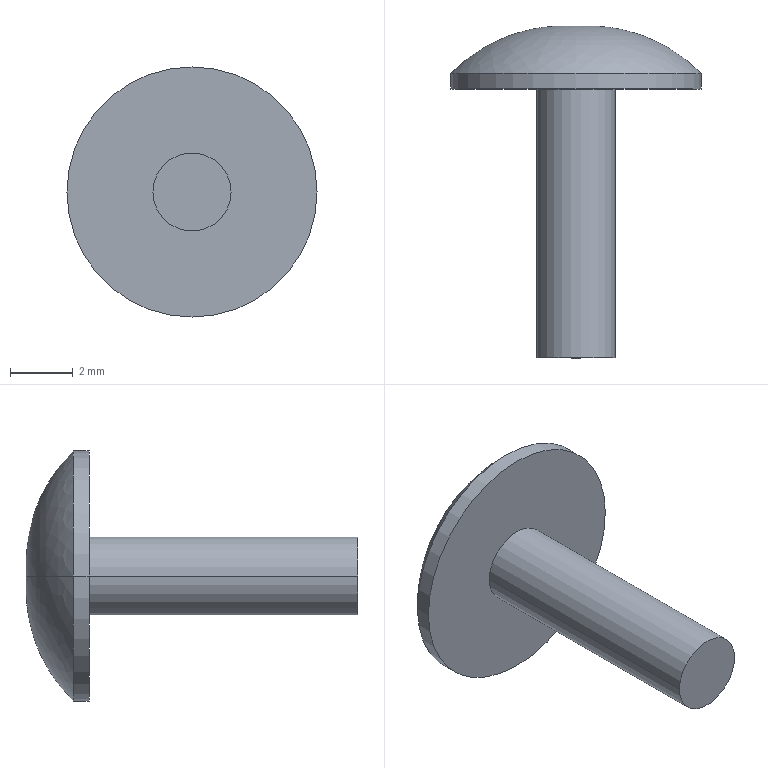Part | STEP file | Glue nail | 1 solid | 8 faces | box 8 x 10.617 x 8 mm | volume 110.388 mm3 | cylinder 4 | other 2 | plane 2 | commonest cylinder face diameters 2.5 x2 8 x2
STEP:
#1=CARTESIAN_POINT('',(0.,0.,0.));
#2=DIRECTION('',(0.,0.,1.));
#3=DIRECTION('',(1.,0.,0.));
#4=AXIS2_PLACEMENT_3D('',#1,#2,#3);
#5=CARTESIAN_POINT('',(-1.25,-10.6,0.));
#6=VERTEX_POINT('',#5);
#7=CARTESIAN_POINT('',(1.25,-10.6,0.));
#8=VERTEX_POINT('',#7);
#9=CARTESIAN_POINT('',(0.,-10.6,0.));
#10=DIRECTION('',(0.,1.,0.));
#11=DIRECTION('',(-1.,0.,0.));
#12=AXIS2_PLACEMENT_3D('',#9,#10,#11);
#13=CIRCLE('',#12,1.25);
#14=CARTESIAN_POINT('',(0.,0.,0.));
#15=DIRECTION('',(0.,1.,0.));
#16=DIRECTION('',(-1.,0.,0.));
#17=AXIS2_PLACEMENT_3D('',#14,#15,#16);
#18=CYLINDRICAL_SURFACE('',#17,1.25);
#19=CARTESIAN_POINT('',(0.,-10.6));
#20=DIRECTION('',(1.,0.));
#21=VECTOR('',#20,1.);
#22=LINE('',#19,#21);
#23=(GEOMETRIC_REPRESENTATION_CONTEXT(2)PARAMETRIC_REPRESENTATION_CONTEXT()REPRESENTATION_CONTEXT('',''));
#24=DEFINITIONAL_REPRESENTATION('',(#22),#23);
#25=PCURVE('',#18,#24);
#26=CARTESIAN_POINT('',(0.,-10.6,0.));
#27=DIRECTION('',(0.,-1.,0.));
#28=DIRECTION('',(1.,0.,0.));
#29=AXIS2_PLACEMENT_3D('',#26,#27,#28);
#30=PLANE('',#29);
#31=CARTESIAN_POINT('',(-1.25,0.));
#32=CARTESIAN_POINT('',(-1.25,2.165));
#33=CARTESIAN_POINT('',(0.625,1.083));
#34=CARTESIAN_POINT('',(2.5,0.));
#35=CARTESIAN_POINT('',(0.625,-1.083));
#36=CARTESIAN_POINT('',(-1.25,-2.165));
#37=CARTESIAN_POINT('',(-1.25,0.));
#38=(BOUNDED_CURVE()B_SPLINE_CURVE(2,(#31,#32,#33,#34,#35,#36,#37),.UNSPECIFIED.,.T.,.F.)B_SPLINE_CURVE_WITH_KNOTS((1,2,2,2,2,1),(-2.094,0.,2.094,4.189,6.283,8.378),.UNSPECIFIED.)CURVE()GEOMETRIC_REPRESENTATION_ITEM()RATIONAL_B_SPLINE_CURVE((1.,0.5,1.,0.5,1.,0.5,1.))REPRESENTATION_ITEM(''));
#39=(GEOMETRIC_REPRESENTATION_CONTEXT(2)PARAMETRIC_REPRESENTATION_CONTEXT()REPRESENTATION_CONTEXT('',''));
#40=DEFINITIONAL_REPRESENTATION('',(#38),#39);
#41=PCURVE('',#30,#40);
#42=SURFACE_CURVE('',#13,(#25,#41),.PCURVE_S1.);
#43=EDGE_CURVE('',#6,#8,#42,.T.);
#44=ORIENTED_EDGE('',*,*,#43,.T.);
#45=CARTESIAN_POINT('',(1.25,-2.,0.));
#46=VERTEX_POINT('',#45);
#47=CARTESIAN_POINT('',(1.25,0.,0.));
#48=DIRECTION('',(0.,1.,0.));
#49=VECTOR('',#48,1.);
#50=LINE('',#47,#49);
#51=CARTESIAN_POINT('',(3.142,0.));
#52=DIRECTION('',(0.,1.));
#53=VECTOR('',#52,1.);
#54=LINE('',#51,#53);
#55=(GEOMETRIC_REPRESENTATION_CONTEXT(2)PARAMETRIC_REPRESENTATION_CONTEXT()REPRESENTATION_CONTEXT('',''));
#56=DEFINITIONAL_REPRESENTATION('',(#54),#55);
#57=PCURVE('',#18,#56);
#58=CARTESIAN_POINT('',(0.,0.,0.));
#59=DIRECTION('',(0.,1.,0.));
#60=DIRECTION('',(-1.,0.,0.));
#61=AXIS2_PLACEMENT_3D('',#58,#59,#60);
#62=CYLINDRICAL_SURFACE('',#61,1.25);
#63=CARTESIAN_POINT('',(3.142,0.));
#64=DIRECTION('',(0.,1.));
#65=VECTOR('',#64,1.);
#66=LINE('',#63,#65);
#67=(GEOMETRIC_REPRESENTATION_CONTEXT(2)PARAMETRIC_REPRESENTATION_CONTEXT()REPRESENTATION_CONTEXT('',''));
#68=DEFINITIONAL_REPRESENTATION('',(#66),#67);
#69=PCURVE('',#62,#68);
#70=SURFACE_CURVE('',#50,(#57,#69),.PCURVE_S1.);
#71=EDGE_CURVE('',#8,#46,#70,.T.);
#72=ORIENTED_EDGE('',*,*,#71,.T.);
#73=CARTESIAN_POINT('',(-1.25,-2.,0.));
#74=VERTEX_POINT('',#73);
#75=CARTESIAN_POINT('',(0.,-2.,0.));
#76=DIRECTION('',(0.,1.,0.));
#77=DIRECTION('',(-1.,0.,0.));
#78=AXIS2_PLACEMENT_3D('',#75,#76,#77);
#79=CIRCLE('',#78,1.25);
#80=CARTESIAN_POINT('',(0.,-2.));
#81=DIRECTION('',(1.,0.));
#82=VECTOR('',#81,1.);
#83=LINE('',#80,#82);
#84=(GEOMETRIC_REPRESENTATION_CONTEXT(2)PARAMETRIC_REPRESENTATION_CONTEXT()REPRESENTATION_CONTEXT('',''));
#85=DEFINITIONAL_REPRESENTATION('',(#83),#84);
#86=PCURVE('',#18,#85);
#87=CARTESIAN_POINT('',(-1.25,-2.,0.));
#88=DIRECTION('',(0.,-1.,0.));
#89=DIRECTION('',(1.,0.,0.));
#90=AXIS2_PLACEMENT_3D('',#87,#88,#89);
#91=PLANE('',#90);
#92=CARTESIAN_POINT('',(0.,0.));
#93=CARTESIAN_POINT('',(0.,2.165));
#94=CARTESIAN_POINT('',(1.875,1.083));
#95=CARTESIAN_POINT('',(3.75,0.));
#96=CARTESIAN_POINT('',(1.875,-1.083));
#97=CARTESIAN_POINT('',(0.,-2.165));
#98=CARTESIAN_POINT('',(0.,0.));
#99=(BOUNDED_CURVE()B_SPLINE_CURVE(2,(#92,#93,#94,#95,#96,#97,#98),.UNSPECIFIED.,.T.,.F.)B_SPLINE_CURVE_WITH_KNOTS((1,2,2,2,2,1),(-2.094,0.,2.094,4.189,6.283,8.378),.UNSPECIFIED.)CURVE()GEOMETRIC_REPRESENTATION_ITEM()RATIONAL_B_SPLINE_CURVE((1.,0.5,1.,0.5,1.,0.5,1.))REPRESENTATION_ITEM(''));
#100=(GEOMETRIC_REPRESENTATION_CONTEXT(2)PARAMETRIC_REPRESENTATION_CONTEXT()REPRESENTATION_CONTEXT('',''));
#101=DEFINITIONAL_REPRESENTATION('',(#99),#100);
#102=PCURVE('',#91,#101);
#103=SURFACE_CURVE('',#79,(#86,#102),.PCURVE_S1.);
#104=EDGE_CURVE('',#74,#46,#103,.T.);
#105=ORIENTED_EDGE('',*,*,#104,.F.);
#106=CARTESIAN_POINT('',(-1.25,0.,0.));
#107=DIRECTION('',(0.,1.,0.));
#108=VECTOR('',#107,1.);
#109=LINE('',#106,#108);
#110=CARTESIAN_POINT('',(0.,0.));
#111=DIRECTION('',(0.,1.));
#112=VECTOR('',#111,1.);
#113=LINE('',#110,#112);
#114=(GEOMETRIC_REPRESENTATION_CONTEXT(2)PARAMETRIC_REPRESENTATION_CONTEXT()REPRESENTATION_CONTEXT('',''));
#115=DEFINITIONAL_REPRESENTATION('',(#113),#114);
#116=PCURVE('',#18,#115);
#117=CARTESIAN_POINT('',(6.283,0.));
#118=DIRECTION('',(0.,1.));
#119=VECTOR('',#118,1.);
#120=LINE('',#117,#119);
#121=(GEOMETRIC_REPRESENTATION_CONTEXT(2)PARAMETRIC_REPRESENTATION_CONTEXT()REPRESENTATION_CONTEXT('',''));
#122=DEFINITIONAL_REPRESENTATION('',(#120),#121);
#123=PCURVE('',#62,#122);
#124=SURFACE_CURVE('',#109,(#116,#123),.PCURVE_S1.);
#125=EDGE_CURVE('',#6,#74,#124,.T.);
#126=ORIENTED_EDGE('',*,*,#125,.F.);
#127=EDGE_LOOP('',(#44,#72,#105,#126));
#128=FACE_BOUND('',#127,.T.);
#129=ADVANCED_FACE('',(#128),#18,.T.);
#130=CARTESIAN_POINT('',(-4.,-2.,0.));
#131=VERTEX_POINT('',#130);
#132=CARTESIAN_POINT('',(4.,-2.,0.));
#133=VERTEX_POINT('',#132);
#134=CARTESIAN_POINT('',(0.,-2.,0.));
#135=DIRECTION('',(0.,1.,0.));
#136=DIRECTION('',(-1.,0.,0.));
#137=AXIS2_PLACEMENT_3D('',#134,#135,#136);
#138=CIRCLE('',#137,4.);
#139=CARTESIAN_POINT('',(0.,0.,0.));
#140=DIRECTION('',(0.,1.,0.));
#141=DIRECTION('',(-1.,0.,0.));
#142=AXIS2_PLACEMENT_3D('',#139,#140,#141);
#143=CYLINDRICAL_SURFACE('',#142,4.);
#144=CARTESIAN_POINT('',(0.,-2.));
#145=DIRECTION('',(1.,0.));
#146=VECTOR('',#145,1.);
#147=LINE('',#144,#146);
#148=(GEOMETRIC_REPRESENTATION_CONTEXT(2)PARAMETRIC_REPRESENTATION_CONTEXT()REPRESENTATION_CONTEXT('',''));
#149=DEFINITIONAL_REPRESENTATION('',(#147),#148);
#150=PCURVE('',#143,#149);
#151=CARTESIAN_POINT('',(-2.75,0.));
#152=CARTESIAN_POINT('',(-2.75,6.928));
#153=CARTESIAN_POINT('',(3.25,3.464));
#154=CARTESIAN_POINT('',(9.25,0.));
#155=CARTESIAN_POINT('',(3.25,-3.464));
#156=CARTESIAN_POINT('',(-2.75,-6.928));
#157=CARTESIAN_POINT('',(-2.75,0.));
#158=(BOUNDED_CURVE()B_SPLINE_CURVE(2,(#151,#152,#153,#154,#155,#156,#157),.UNSPECIFIED.,.T.,.F.)B_SPLINE_CURVE_WITH_KNOTS((1,2,2,2,2,1),(-2.094,0.,2.094,4.189,6.283,8.378),.UNSPECIFIED.)CURVE()GEOMETRIC_REPRESENTATION_ITEM()RATIONAL_B_SPLINE_CURVE((1.,0.5,1.,0.5,1.,0.5,1.))REPRESENTATION_ITEM(''));
#159=(GEOMETRIC_REPRESENTATION_CONTEXT(2)PARAMETRIC_REPRESENTATION_CONTEXT()REPRESENTATION_CONTEXT('',''));
#160=DEFINITIONAL_REPRESENTATION('',(#158),#159);
#161=PCURVE('',#91,#160);
#162=SURFACE_CURVE('',#138,(#150,#161),.PCURVE_S1.);
#163=EDGE_CURVE('',#131,#133,#162,.T.);
#164=ORIENTED_EDGE('',*,*,#163,.T.);
#165=CARTESIAN_POINT('',(4.,-1.5,0.));
#166=VERTEX_POINT('',#165);
#167=CARTESIAN_POINT('',(4.,0.,0.));
#168=DIRECTION('',(0.,1.,0.));
#169=VECTOR('',#168,1.);
#170=LINE('',#167,#169);
#171=CARTESIAN_POINT('',(3.142,0.));
#172=DIRECTION('',(0.,1.));
#173=VECTOR('',#172,1.);
#174=LINE('',#171,#173);
#175=(GEOMETRIC_REPRESENTATION_CONTEXT(2)PARAMETRIC_REPRESENTATION_CONTEXT()REPRESENTATION_CONTEXT('',''));
#176=DEFINITIONAL_REPRESENTATION('',(#174),#175);
#177=PCURVE('',#143,#176);
#178=CARTESIAN_POINT('',(0.,0.,0.));
#179=DIRECTION('',(0.,1.,0.));
#180=DIRECTION('',(-1.,0.,0.));
#181=AXIS2_PLACEMENT_3D('',#178,#179,#180);
#182=CYLINDRICAL_SURFACE('',#181,4.);
#183=CARTESIAN_POINT('',(3.142,0.));
#184=DIRECTION('',(0.,1.));
#185=VECTOR('',#184,1.);
#186=LINE('',#183,#185);
#187=(GEOMETRIC_REPRESENTATION_CONTEXT(2)PARAMETRIC_REPRESENTATION_CONTEXT()REPRESENTATION_CONTEXT('',''));
#188=DEFINITIONAL_REPRESENTATION('',(#186),#187);
#189=PCURVE('',#182,#188);
#190=SURFACE_CURVE('',#170,(#177,#189),.PCURVE_S1.);
#191=EDGE_CURVE('',#133,#166,#190,.T.);
#192=ORIENTED_EDGE('',*,*,#191,.T.);
#193=CARTESIAN_POINT('',(-4.,-1.5,0.));
#194=VERTEX_POINT('',#193);
#195=CARTESIAN_POINT('',(0.,-1.5,0.));
#196=DIRECTION('',(0.,1.,0.));
#197=DIRECTION('',(-1.,0.,0.));
#198=AXIS2_PLACEMENT_3D('',#195,#196,#197);
#199=CIRCLE('',#198,4.);
#200=CARTESIAN_POINT('',(0.,-1.5));
#201=DIRECTION('',(1.,0.));
#202=VECTOR('',#201,1.);
#203=LINE('',#200,#202);
#204=(GEOMETRIC_REPRESENTATION_CONTEXT(2)PARAMETRIC_REPRESENTATION_CONTEXT()REPRESENTATION_CONTEXT('',''));
#205=DEFINITIONAL_REPRESENTATION('',(#203),#204);
#206=PCURVE('',#143,#205);
#207=CARTESIAN_POINT('',(-4.,-1.5,0.));
#208=CARTESIAN_POINT('',(-3.488,-0.9722,0.));
#209=CARTESIAN_POINT('',(-2.882,-0.5349,0.));
#210=CARTESIAN_POINT('',(-2.203,-0.2086,0.));
#211=CARTESIAN_POINT('',(-1.477,-0.008015,0.));
#212=CARTESIAN_POINT('',(-0.7331,0.06071,0.));
#213=CARTESIAN_POINT('',(0.,0.,0.));
#214=B_SPLINE_CURVE_WITH_KNOTS('',6,(#207,#208,#209,#210,#211,#212,#213),.UNSPECIFIED.,.F.,.F.,(7,7),(0.7706,1.653),.PIECEWISE_BEZIER_KNOTS.);
#215=CARTESIAN_POINT('',(0.,-4.983,0.));
#216=DIRECTION('',(0.,1.,0.));
#217=AXIS1_PLACEMENT('',#215,#216);
#218=SURFACE_OF_REVOLUTION('',#214,#217);
#219=CARTESIAN_POINT('',(0.,0.7706));
#220=DIRECTION('',(1.,0.));
#221=VECTOR('',#220,1.);
#222=LINE('',#219,#221);
#223=(GEOMETRIC_REPRESENTATION_CONTEXT(2)PARAMETRIC_REPRESENTATION_CONTEXT()REPRESENTATION_CONTEXT('',''));
#224=DEFINITIONAL_REPRESENTATION('',(#222),#223);
#225=PCURVE('',#218,#224);
#226=SURFACE_CURVE('',#199,(#206,#225),.PCURVE_S1.);
#227=EDGE_CURVE('',#194,#166,#226,.T.);
#228=ORIENTED_EDGE('',*,*,#227,.F.);
#229=CARTESIAN_POINT('',(-4.,0.,0.));
#230=DIRECTION('',(0.,1.,0.));
#231=VECTOR('',#230,1.);
#232=LINE('',#229,#231);
#233=CARTESIAN_POINT('',(0.,0.));
#234=DIRECTION('',(0.,1.));
#235=VECTOR('',#234,1.);
#236=LINE('',#233,#235);
#237=(GEOMETRIC_REPRESENTATION_CONTEXT(2)PARAMETRIC_REPRESENTATION_CONTEXT()REPRESENTATION_CONTEXT('',''));
#238=DEFINITIONAL_REPRESENTATION('',(#236),#237);
#239=PCURVE('',#143,#238);
#240=CARTESIAN_POINT('',(6.283,0.));
#241=DIRECTION('',(0.,1.));
#242=VECTOR('',#241,1.);
#243=LINE('',#240,#242);
#244=(GEOMETRIC_REPRESENTATION_CONTEXT(2)PARAMETRIC_REPRESENTATION_CONTEXT()REPRESENTATION_CONTEXT('',''));
#245=DEFINITIONAL_REPRESENTATION('',(#243),#244);
#246=PCURVE('',#182,#245);
#247=SURFACE_CURVE('',#232,(#239,#246),.PCURVE_S1.);
#248=EDGE_CURVE('',#131,#194,#247,.T.);
#249=ORIENTED_EDGE('',*,*,#248,.F.);
#250=EDGE_LOOP('',(#164,#192,#228,#249));
#251=FACE_BOUND('',#250,.T.);
#252=ADVANCED_FACE('',(#251),#143,.T.);
#253=ORIENTED_EDGE('',*,*,#227,.T.);
#254=CARTESIAN_POINT('',(0.,0.,0.));
#255=VERTEX_POINT('',#254);
#256=CARTESIAN_POINT('',(0.4126,-4.983,0.));
#257=DIRECTION('',(0.,0.,1.));
#258=DIRECTION('',(1.,0.,0.));
#259=AXIS2_PLACEMENT_3D('',#256,#257,#258);
#260=CIRCLE('',#259,5.);
#261=CARTESIAN_POINT('',(3.142,0.7706));
#262=CARTESIAN_POINT('',(3.142,0.784));
#263=CARTESIAN_POINT('',(3.142,0.8108));
#264=CARTESIAN_POINT('',(3.142,0.8509));
#265=CARTESIAN_POINT('',(3.142,0.891));
#266=CARTESIAN_POINT('',(3.142,0.9311));
#267=CARTESIAN_POINT('',(3.142,0.9713));
#268=CARTESIAN_POINT('',(3.142,1.011));
#269=CARTESIAN_POINT('',(3.142,1.052));
#270=CARTESIAN_POINT('',(3.142,1.092));
#271=CARTESIAN_POINT('',(3.142,1.132));
#272=CARTESIAN_POINT('',(3.142,1.172));
#273=CARTESIAN_POINT('',(3.142,1.212));
#274=CARTESIAN_POINT('',(3.142,1.252));
#275=CARTESIAN_POINT('',(3.142,1.292));
#276=CARTESIAN_POINT('',(3.142,1.332));
#277=CARTESIAN_POINT('',(3.142,1.373));
#278=CARTESIAN_POINT('',(3.142,1.413));
#279=CARTESIAN_POINT('',(3.142,1.453));
#280=CARTESIAN_POINT('',(3.142,1.493));
#281=CARTESIAN_POINT('',(3.142,1.533));
#282=CARTESIAN_POINT('',(3.142,1.573));
#283=CARTESIAN_POINT('',(3.142,1.613));
#284=CARTESIAN_POINT('',(3.142,1.64));
#285=CARTESIAN_POINT('',(3.142,1.653));
#286=B_SPLINE_CURVE_WITH_KNOTS('',3,(#261,#262,#263,#264,#265,#266,#267,#268,#269,#270,#271,#272,#273,#274,#275,#276,#277,#278,#279,#280,#281,#282,#283,#284,#285),.UNSPECIFIED.,.F.,.F.,(4,1,1,1,1,1,1,1,1,1,1,1,1,1,1,1,1,1,1,1,1,1,4),(0.7706,0.8108,0.8509,0.891,0.9311,0.9713,1.011,1.052,1.092,1.132,1.172,1.212,1.252,1.292,1.332,1.373,1.413,1.453,1.493,1.533,1.573,1.613,1.653),.QUASI_UNIFORM_KNOTS.);
#287=(GEOMETRIC_REPRESENTATION_CONTEXT(2)PARAMETRIC_REPRESENTATION_CONTEXT()REPRESENTATION_CONTEXT('',''));
#288=DEFINITIONAL_REPRESENTATION('',(#286),#287);
#289=PCURVE('',#218,#288);
#290=CARTESIAN_POINT('',(-4.,-1.5,0.));
#291=CARTESIAN_POINT('',(-3.488,-0.9722,0.));
#292=CARTESIAN_POINT('',(-2.882,-0.5349,0.));
#293=CARTESIAN_POINT('',(-2.203,-0.2086,0.));
#294=CARTESIAN_POINT('',(-1.477,-0.008015,0.));
#295=CARTESIAN_POINT('',(-0.7331,0.06071,0.));
#296=CARTESIAN_POINT('',(0.,0.,0.));
#297=B_SPLINE_CURVE_WITH_KNOTS('',6,(#290,#291,#292,#293,#294,#295,#296),.UNSPECIFIED.,.F.,.F.,(7,7),(0.7706,1.653),.PIECEWISE_BEZIER_KNOTS.);
#298=CARTESIAN_POINT('',(0.,-4.983,0.));
#299=DIRECTION('',(0.,1.,0.));
#300=AXIS1_PLACEMENT('',#298,#299);
#301=SURFACE_OF_REVOLUTION('',#297,#300);
#302=CARTESIAN_POINT('',(3.142,0.7706));
#303=CARTESIAN_POINT('',(3.142,0.784));
#304=CARTESIAN_POINT('',(3.142,0.8108));
#305=CARTESIAN_POINT('',(3.142,0.8509));
#306=CARTESIAN_POINT('',(3.142,0.891));
#307=CARTESIAN_POINT('',(3.142,0.9311));
#308=CARTESIAN_POINT('',(3.142,0.9713));
#309=CARTESIAN_POINT('',(3.142,1.011));
#310=CARTESIAN_POINT('',(3.142,1.052));
#311=CARTESIAN_POINT('',(3.142,1.092));
#312=CARTESIAN_POINT('',(3.142,1.132));
#313=CARTESIAN_POINT('',(3.142,1.172));
#314=CARTESIAN_POINT('',(3.142,1.212));
#315=CARTESIAN_POINT('',(3.142,1.252));
#316=CARTESIAN_POINT('',(3.142,1.292));
#317=CARTESIAN_POINT('',(3.142,1.332));
#318=CARTESIAN_POINT('',(3.142,1.373));
#319=CARTESIAN_POINT('',(3.142,1.413));
#320=CARTESIAN_POINT('',(3.142,1.453));
#321=CARTESIAN_POINT('',(3.142,1.493));
#322=CARTESIAN_POINT('',(3.142,1.533));
#323=CARTESIAN_POINT('',(3.142,1.573));
#324=CARTESIAN_POINT('',(3.142,1.613));
#325=CARTESIAN_POINT('',(3.142,1.64));
#326=CARTESIAN_POINT('',(3.142,1.653));
#327=B_SPLINE_CURVE_WITH_KNOTS('',3,(#302,#303,#304,#305,#306,#307,#308,#309,#310,#311,#312,#313,#314,#315,#316,#317,#318,#319,#320,#321,#322,#323,#324,#325,#326),.UNSPECIFIED.,.F.,.F.,(4,1,1,1,1,1,1,1,1,1,1,1,1,1,1,1,1,1,1,1,1,1,4),(0.7706,0.8108,0.8509,0.891,0.9311,0.9713,1.011,1.052,1.092,1.132,1.172,1.212,1.252,1.292,1.332,1.373,1.413,1.453,1.493,1.533,1.573,1.613,1.653),.QUASI_UNIFORM_KNOTS.);
#328=(GEOMETRIC_REPRESENTATION_CONTEXT(2)PARAMETRIC_REPRESENTATION_CONTEXT()REPRESENTATION_CONTEXT('',''));
#329=DEFINITIONAL_REPRESENTATION('',(#327),#328);
#330=PCURVE('',#301,#329);
#331=SURFACE_CURVE('',#260,(#289,#330),.PCURVE_S1.);
#332=EDGE_CURVE('',#166,#255,#331,.T.);
#333=ORIENTED_EDGE('',*,*,#332,.T.);
#334=CARTESIAN_POINT('',(-0.4126,-4.983,0.));
#335=DIRECTION('',(0.,0.,-1.));
#336=DIRECTION('',(-1.,0.,0.));
#337=AXIS2_PLACEMENT_3D('',#334,#335,#336);
#338=CIRCLE('',#337,5.);
#339=CARTESIAN_POINT('',(0.,0.7706));
#340=CARTESIAN_POINT('',(0.,0.784));
#341=CARTESIAN_POINT('',(0.,0.8108));
#342=CARTESIAN_POINT('',(0.,0.8509));
#343=CARTESIAN_POINT('',(0.,0.891));
#344=CARTESIAN_POINT('',(0.,0.9311));
#345=CARTESIAN_POINT('',(0.,0.9713));
#346=CARTESIAN_POINT('',(0.,1.011));
#347=CARTESIAN_POINT('',(0.,1.052));
#348=CARTESIAN_POINT('',(0.,1.092));
#349=CARTESIAN_POINT('',(0.,1.132));
#350=CARTESIAN_POINT('',(0.,1.172));
#351=CARTESIAN_POINT('',(0.,1.212));
#352=CARTESIAN_POINT('',(0.,1.252));
#353=CARTESIAN_POINT('',(0.,1.292));
#354=CARTESIAN_POINT('',(0.,1.332));
#355=CARTESIAN_POINT('',(0.,1.373));
#356=CARTESIAN_POINT('',(0.,1.413));
#357=CARTESIAN_POINT('',(0.,1.453));
#358=CARTESIAN_POINT('',(0.,1.493));
#359=CARTESIAN_POINT('',(0.,1.533));
#360=CARTESIAN_POINT('',(0.,1.573));
#361=CARTESIAN_POINT('',(0.,1.613));
#362=CARTESIAN_POINT('',(0.,1.64));
#363=CARTESIAN_POINT('',(0.,1.653));
#364=B_SPLINE_CURVE_WITH_KNOTS('',3,(#339,#340,#341,#342,#343,#344,#345,#346,#347,#348,#349,#350,#351,#352,#353,#354,#355,#356,#357,#358,#359,#360,#361,#362,#363),.UNSPECIFIED.,.F.,.F.,(4,1,1,1,1,1,1,1,1,1,1,1,1,1,1,1,1,1,1,1,1,1,4),(0.7706,0.8108,0.8509,0.891,0.9311,0.9713,1.011,1.052,1.092,1.132,1.172,1.212,1.252,1.292,1.332,1.373,1.413,1.453,1.493,1.533,1.573,1.613,1.653),.QUASI_UNIFORM_KNOTS.);
#365=(GEOMETRIC_REPRESENTATION_CONTEXT(2)PARAMETRIC_REPRESENTATION_CONTEXT()REPRESENTATION_CONTEXT('',''));
#366=DEFINITIONAL_REPRESENTATION('',(#364),#365);
#367=PCURVE('',#218,#366);
#368=CARTESIAN_POINT('',(6.283,0.7706));
#369=CARTESIAN_POINT('',(6.283,0.784));
#370=CARTESIAN_POINT('',(6.283,0.8108));
#371=CARTESIAN_POINT('',(6.283,0.8509));
#372=CARTESIAN_POINT('',(6.283,0.891));
#373=CARTESIAN_POINT('',(6.283,0.9311));
#374=CARTESIAN_POINT('',(6.283,0.9713));
#375=CARTESIAN_POINT('',(6.283,1.011));
#376=CARTESIAN_POINT('',(6.283,1.052));
#377=CARTESIAN_POINT('',(6.283,1.092));
#378=CARTESIAN_POINT('',(6.283,1.132));
#379=CARTESIAN_POINT('',(6.283,1.172));
#380=CARTESIAN_POINT('',(6.283,1.212));
#381=CARTESIAN_POINT('',(6.283,1.252));
#382=CARTESIAN_POINT('',(6.283,1.292));
#383=CARTESIAN_POINT('',(6.283,1.332));
#384=CARTESIAN_POINT('',(6.283,1.373));
#385=CARTESIAN_POINT('',(6.283,1.413));
#386=CARTESIAN_POINT('',(6.283,1.453));
#387=CARTESIAN_POINT('',(6.283,1.493));
#388=CARTESIAN_POINT('',(6.283,1.533));
#389=CARTESIAN_POINT('',(6.283,1.573));
#390=CARTESIAN_POINT('',(6.283,1.613));
#391=CARTESIAN_POINT('',(6.283,1.64));
#392=CARTESIAN_POINT('',(6.283,1.653));
#393=B_SPLINE_CURVE_WITH_KNOTS('',3,(#368,#369,#370,#371,#372,#373,#374,#375,#376,#377,#378,#379,#380,#381,#382,#383,#384,#385,#386,#387,#388,#389,#390,#391,#392),.UNSPECIFIED.,.F.,.F.,(4,1,1,1,1,1,1,1,1,1,1,1,1,1,1,1,1,1,1,1,1,1,4),(0.7706,0.8108,0.8509,0.891,0.9311,0.9713,1.011,1.052,1.092,1.132,1.172,1.212,1.252,1.292,1.332,1.373,1.413,1.453,1.493,1.533,1.573,1.613,1.653),.QUASI_UNIFORM_KNOTS.);
#394=(GEOMETRIC_REPRESENTATION_CONTEXT(2)PARAMETRIC_REPRESENTATION_CONTEXT()REPRESENTATION_CONTEXT('',''));
#395=DEFINITIONAL_REPRESENTATION('',(#393),#394);
#396=PCURVE('',#301,#395);
#397=SURFACE_CURVE('',#338,(#367,#396),.PCURVE_S1.);
#398=EDGE_CURVE('',#194,#255,#397,.T.);
#399=ORIENTED_EDGE('',*,*,#398,.F.);
#400=EDGE_LOOP('',(#253,#333,#399));
#401=FACE_BOUND('',#400,.T.);
#402=ADVANCED_FACE('',(#401),#218,.T.);
#403=ORIENTED_EDGE('',*,*,#332,.F.);
#404=CARTESIAN_POINT('',(0.,-1.5,0.));
#405=DIRECTION('',(0.,1.,0.));
#406=DIRECTION('',(-1.,0.,0.));
#407=AXIS2_PLACEMENT_3D('',#404,#405,#406);
#408=CIRCLE('',#407,4.);
#409=CARTESIAN_POINT('',(0.,0.7706));
#410=DIRECTION('',(1.,0.));
#411=VECTOR('',#410,1.);
#412=LINE('',#409,#411);
#413=(GEOMETRIC_REPRESENTATION_CONTEXT(2)PARAMETRIC_REPRESENTATION_CONTEXT()REPRESENTATION_CONTEXT('',''));
#414=DEFINITIONAL_REPRESENTATION('',(#412),#413);
#415=PCURVE('',#301,#414);
#416=CARTESIAN_POINT('',(0.,-1.5));
#417=DIRECTION('',(1.,0.));
#418=VECTOR('',#417,1.);
#419=LINE('',#416,#418);
#420=(GEOMETRIC_REPRESENTATION_CONTEXT(2)PARAMETRIC_REPRESENTATION_CONTEXT()REPRESENTATION_CONTEXT('',''));
#421=DEFINITIONAL_REPRESENTATION('',(#419),#420);
#422=PCURVE('',#182,#421);
#423=SURFACE_CURVE('',#408,(#415,#422),.PCURVE_S1.);
#424=EDGE_CURVE('',#166,#194,#423,.T.);
#425=ORIENTED_EDGE('',*,*,#424,.T.);
#426=ORIENTED_EDGE('',*,*,#398,.T.);
#427=EDGE_LOOP('',(#403,#425,#426));
#428=FACE_BOUND('',#427,.T.);
#429=ADVANCED_FACE('',(#428),#301,.T.);
#430=ORIENTED_EDGE('',*,*,#191,.F.);
#431=CARTESIAN_POINT('',(0.,-2.,0.));
#432=DIRECTION('',(0.,1.,0.));
#433=DIRECTION('',(-1.,0.,0.));
#434=AXIS2_PLACEMENT_3D('',#431,#432,#433);
#435=CIRCLE('',#434,4.);
#436=CARTESIAN_POINT('',(0.,-2.));
#437=DIRECTION('',(1.,0.));
#438=VECTOR('',#437,1.);
#439=LINE('',#436,#438);
#440=(GEOMETRIC_REPRESENTATION_CONTEXT(2)PARAMETRIC_REPRESENTATION_CONTEXT()REPRESENTATION_CONTEXT('',''));
#441=DEFINITIONAL_REPRESENTATION('',(#439),#440);
#442=PCURVE('',#182,#441);
#443=CARTESIAN_POINT('',(-2.75,0.));
#444=CARTESIAN_POINT('',(-2.75,6.928));
#445=CARTESIAN_POINT('',(3.25,3.464));
#446=CARTESIAN_POINT('',(9.25,0.));
#447=CARTESIAN_POINT('',(3.25,-3.464));
#448=CARTESIAN_POINT('',(-2.75,-6.928));
#449=CARTESIAN_POINT('',(-2.75,0.));
#450=(BOUNDED_CURVE()B_SPLINE_CURVE(2,(#443,#444,#445,#446,#447,#448,#449),.UNSPECIFIED.,.T.,.F.)B_SPLINE_CURVE_WITH_KNOTS((1,2,2,2,2,1),(-2.094,0.,2.094,4.189,6.283,8.378),.UNSPECIFIED.)CURVE()GEOMETRIC_REPRESENTATION_ITEM()RATIONAL_B_SPLINE_CURVE((1.,0.5,1.,0.5,1.,0.5,1.))REPRESENTATION_ITEM(''));
#451=(GEOMETRIC_REPRESENTATION_CONTEXT(2)PARAMETRIC_REPRESENTATION_CONTEXT()REPRESENTATION_CONTEXT('',''));
#452=DEFINITIONAL_REPRESENTATION('',(#450),#451);
#453=PCURVE('',#91,#452);
#454=SURFACE_CURVE('',#435,(#442,#453),.PCURVE_S1.);
#455=EDGE_CURVE('',#133,#131,#454,.T.);
#456=ORIENTED_EDGE('',*,*,#455,.T.);
#457=ORIENTED_EDGE('',*,*,#248,.T.);
#458=ORIENTED_EDGE('',*,*,#424,.F.);
#459=EDGE_LOOP('',(#430,#456,#457,#458));
#460=FACE_BOUND('',#459,.T.);
#461=ADVANCED_FACE('',(#460),#182,.T.);
#462=ORIENTED_EDGE('',*,*,#104,.T.);
#463=CARTESIAN_POINT('',(0.,-2.,0.));
#464=DIRECTION('',(0.,1.,0.));
#465=DIRECTION('',(-1.,0.,0.));
#466=AXIS2_PLACEMENT_3D('',#463,#464,#465);
#467=CIRCLE('',#466,1.25);
#468=CARTESIAN_POINT('',(0.,0.));
#469=CARTESIAN_POINT('',(0.,2.165));
#470=CARTESIAN_POINT('',(1.875,1.083));
#471=CARTESIAN_POINT('',(3.75,0.));
#472=CARTESIAN_POINT('',(1.875,-1.083));
#473=CARTESIAN_POINT('',(0.,-2.165));
#474=CARTESIAN_POINT('',(0.,0.));
#475=(BOUNDED_CURVE()B_SPLINE_CURVE(2,(#468,#469,#470,#471,#472,#473,#474),.UNSPECIFIED.,.T.,.F.)B_SPLINE_CURVE_WITH_KNOTS((1,2,2,2,2,1),(-2.094,0.,2.094,4.189,6.283,8.378),.UNSPECIFIED.)CURVE()GEOMETRIC_REPRESENTATION_ITEM()RATIONAL_B_SPLINE_CURVE((1.,0.5,1.,0.5,1.,0.5,1.))REPRESENTATION_ITEM(''));
#476=(GEOMETRIC_REPRESENTATION_CONTEXT(2)PARAMETRIC_REPRESENTATION_CONTEXT()REPRESENTATION_CONTEXT('',''));
#477=DEFINITIONAL_REPRESENTATION('',(#475),#476);
#478=PCURVE('',#91,#477);
#479=CARTESIAN_POINT('',(0.,-2.));
#480=DIRECTION('',(1.,0.));
#481=VECTOR('',#480,1.);
#482=LINE('',#479,#481);
#483=(GEOMETRIC_REPRESENTATION_CONTEXT(2)PARAMETRIC_REPRESENTATION_CONTEXT()REPRESENTATION_CONTEXT('',''));
#484=DEFINITIONAL_REPRESENTATION('',(#482),#483);
#485=PCURVE('',#62,#484);
#486=SURFACE_CURVE('',#467,(#478,#485),.PCURVE_S1.);
#487=EDGE_CURVE('',#46,#74,#486,.T.);
#488=ORIENTED_EDGE('',*,*,#487,.T.);
#489=EDGE_LOOP('',(#462,#488));
#490=FACE_BOUND('',#489,.T.);
#491=ORIENTED_EDGE('',*,*,#163,.F.);
#492=ORIENTED_EDGE('',*,*,#455,.F.);
#493=EDGE_LOOP('',(#491,#492));
#494=FACE_BOUND('',#493,.T.);
#495=ADVANCED_FACE('',(#490,#494),#91,.T.);
#496=ORIENTED_EDGE('',*,*,#71,.F.);
#497=CARTESIAN_POINT('',(0.,-10.6,0.));
#498=DIRECTION('',(0.,1.,0.));
#499=DIRECTION('',(-1.,0.,0.));
#500=AXIS2_PLACEMENT_3D('',#497,#498,#499);
#501=CIRCLE('',#500,1.25);
#502=CARTESIAN_POINT('',(0.,-10.6));
#503=DIRECTION('',(1.,0.));
#504=VECTOR('',#503,1.);
#505=LINE('',#502,#504);
#506=(GEOMETRIC_REPRESENTATION_CONTEXT(2)PARAMETRIC_REPRESENTATION_CONTEXT()REPRESENTATION_CONTEXT('',''));
#507=DEFINITIONAL_REPRESENTATION('',(#505),#506);
#508=PCURVE('',#62,#507);
#509=CARTESIAN_POINT('',(-1.25,0.));
#510=CARTESIAN_POINT('',(-1.25,2.165));
#511=CARTESIAN_POINT('',(0.625,1.083));
#512=CARTESIAN_POINT('',(2.5,0.));
#513=CARTESIAN_POINT('',(0.625,-1.083));
#514=CARTESIAN_POINT('',(-1.25,-2.165));
#515=CARTESIAN_POINT('',(-1.25,0.));
#516=(BOUNDED_CURVE()B_SPLINE_CURVE(2,(#509,#510,#511,#512,#513,#514,#515),.UNSPECIFIED.,.T.,.F.)B_SPLINE_CURVE_WITH_KNOTS((1,2,2,2,2,1),(-2.094,0.,2.094,4.189,6.283,8.378),.UNSPECIFIED.)CURVE()GEOMETRIC_REPRESENTATION_ITEM()RATIONAL_B_SPLINE_CURVE((1.,0.5,1.,0.5,1.,0.5,1.))REPRESENTATION_ITEM(''));
#517=(GEOMETRIC_REPRESENTATION_CONTEXT(2)PARAMETRIC_REPRESENTATION_CONTEXT()REPRESENTATION_CONTEXT('',''));
#518=DEFINITIONAL_REPRESENTATION('',(#516),#517);
#519=PCURVE('',#30,#518);
#520=SURFACE_CURVE('',#501,(#508,#519),.PCURVE_S1.);
#521=EDGE_CURVE('',#8,#6,#520,.T.);
#522=ORIENTED_EDGE('',*,*,#521,.T.);
#523=ORIENTED_EDGE('',*,*,#125,.T.);
#524=ORIENTED_EDGE('',*,*,#487,.F.);
#525=EDGE_LOOP('',(#496,#522,#523,#524));
#526=FACE_BOUND('',#525,.T.);
#527=ADVANCED_FACE('',(#526),#62,.T.);
#528=ORIENTED_EDGE('',*,*,#43,.F.);
#529=ORIENTED_EDGE('',*,*,#521,.F.);
#530=EDGE_LOOP('',(#528,#529));
#531=FACE_BOUND('',#530,.T.);
#532=ADVANCED_FACE('',(#531),#30,.T.);
#533=CLOSED_SHELL('',(#129,#252,#402,#429,#461,#495,#527,#532));
#534=MANIFOLD_SOLID_BREP('',#533);
#535=(LENGTH_UNIT()NAMED_UNIT(*)SI_UNIT(.MILLI.,.METRE.));
#536=UNCERTAINTY_MEASURE_WITH_UNIT(LENGTH_MEASURE(0.0000001),#535,'','');
#537=(NAMED_UNIT(*)PLANE_ANGLE_UNIT()SI_UNIT($,.RADIAN.));
#538=(NAMED_UNIT(*)SI_UNIT($,.STERADIAN.)SOLID_ANGLE_UNIT());
#539=(GEOMETRIC_REPRESENTATION_CONTEXT(3)GLOBAL_UNCERTAINTY_ASSIGNED_CONTEXT((#536))GLOBAL_UNIT_ASSIGNED_CONTEXT((#535,#537,#538))REPRESENTATION_CONTEXT('',''));
#540=ADVANCED_BREP_SHAPE_REPRESENTATION('',(#4,#534),#539);